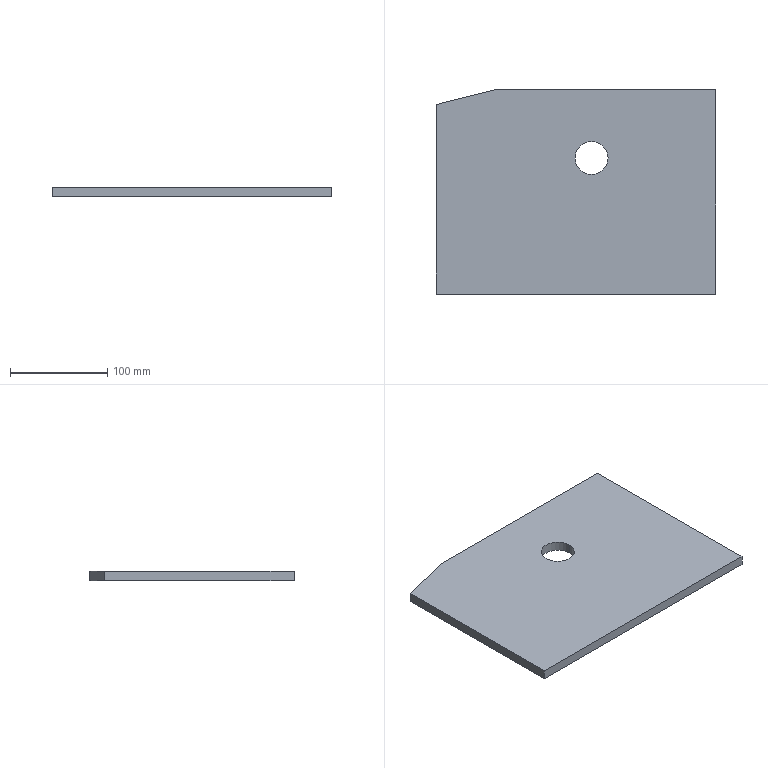Part | STEP file | 001-003-Shaft storage magazine side plate | 1 solid | 9 faces | box 288 x 210 x 10 mm | volume 591209 mm3 | plane 7 | cylinder 2 | commonest cylinder face diameters 34 x2
STEP:
#1=CARTESIAN_POINT('',(0.,0.,0.));
#2=DIRECTION('',(0.,0.,1.));
#3=DIRECTION('',(1.,0.,0.));
#4=AXIS2_PLACEMENT_3D('',#1,#2,#3);
#5=CARTESIAN_POINT('',(-1.,35.,10.));
#6=VERTEX_POINT('',#5);
#7=CARTESIAN_POINT('',(-1.,35.,0.));
#8=VERTEX_POINT('',#7);
#9=CARTESIAN_POINT('',(-1.,35.,10.));
#10=DIRECTION('',(0.,0.,-1.));
#11=VECTOR('',#10,1.);
#12=LINE('',#9,#11);
#13=CARTESIAN_POINT('',(16.,35.,10.));
#14=DIRECTION('',(0.,0.,-1.));
#15=DIRECTION('',(-1.,0.,0.));
#16=AXIS2_PLACEMENT_3D('',#13,#14,#15);
#17=CYLINDRICAL_SURFACE('',#16,17.);
#18=CARTESIAN_POINT('',(6.283,0.));
#19=DIRECTION('',(0.,1.));
#20=VECTOR('',#19,1.);
#21=LINE('',#18,#20);
#22=(GEOMETRIC_REPRESENTATION_CONTEXT(2)PARAMETRIC_REPRESENTATION_CONTEXT()REPRESENTATION_CONTEXT('',''));
#23=DEFINITIONAL_REPRESENTATION('',(#21),#22);
#24=PCURVE('',#17,#23);
#25=CARTESIAN_POINT('',(16.,35.,10.));
#26=DIRECTION('',(0.,0.,-1.));
#27=DIRECTION('',(-1.,0.,0.));
#28=AXIS2_PLACEMENT_3D('',#25,#26,#27);
#29=CYLINDRICAL_SURFACE('',#28,17.);
#30=CARTESIAN_POINT('',(0.,0.));
#31=DIRECTION('',(0.,1.));
#32=VECTOR('',#31,1.);
#33=LINE('',#30,#32);
#34=(GEOMETRIC_REPRESENTATION_CONTEXT(2)PARAMETRIC_REPRESENTATION_CONTEXT()REPRESENTATION_CONTEXT('',''));
#35=DEFINITIONAL_REPRESENTATION('',(#33),#34);
#36=PCURVE('',#29,#35);
#37=SURFACE_CURVE('',#12,(#24,#36),.PCURVE_S1.);
#38=EDGE_CURVE('',#6,#8,#37,.T.);
#39=ORIENTED_EDGE('',*,*,#38,.T.);
#40=CARTESIAN_POINT('',(33.,35.,0.));
#41=VERTEX_POINT('',#40);
#42=CARTESIAN_POINT('',(16.,35.,0.));
#43=DIRECTION('',(0.,0.,-1.));
#44=DIRECTION('',(-1.,0.,0.));
#45=AXIS2_PLACEMENT_3D('',#42,#43,#44);
#46=CIRCLE('',#45,17.);
#47=CARTESIAN_POINT('',(0.,10.));
#48=DIRECTION('',(1.,0.));
#49=VECTOR('',#48,1.);
#50=LINE('',#47,#49);
#51=(GEOMETRIC_REPRESENTATION_CONTEXT(2)PARAMETRIC_REPRESENTATION_CONTEXT()REPRESENTATION_CONTEXT('',''));
#52=DEFINITIONAL_REPRESENTATION('',(#50),#51);
#53=PCURVE('',#17,#52);
#54=CARTESIAN_POINT('',(0.,0.,0.));
#55=DIRECTION('',(0.,0.,-1.));
#56=DIRECTION('',(-1.,0.,0.));
#57=AXIS2_PLACEMENT_3D('',#54,#55,#56);
#58=PLANE('',#57);
#59=CARTESIAN_POINT('',(-16.,35.));
#60=DIRECTION('',(1.,0.));
#61=AXIS2_PLACEMENT_2D('',#59,#60);
#62=CIRCLE('',#61,17.);
#63=(GEOMETRIC_REPRESENTATION_CONTEXT(2)PARAMETRIC_REPRESENTATION_CONTEXT()REPRESENTATION_CONTEXT('',''));
#64=DEFINITIONAL_REPRESENTATION('',(#62),#63);
#65=PCURVE('',#58,#64);
#66=SURFACE_CURVE('',#46,(#53,#65),.PCURVE_S1.);
#67=EDGE_CURVE('',#41,#8,#66,.T.);
#68=ORIENTED_EDGE('',*,*,#67,.F.);
#69=CARTESIAN_POINT('',(33.,35.,10.));
#70=VERTEX_POINT('',#69);
#71=CARTESIAN_POINT('',(33.,35.,10.));
#72=DIRECTION('',(0.,0.,-1.));
#73=VECTOR('',#72,1.);
#74=LINE('',#71,#73);
#75=CARTESIAN_POINT('',(3.142,0.));
#76=DIRECTION('',(0.,1.));
#77=VECTOR('',#76,1.);
#78=LINE('',#75,#77);
#79=(GEOMETRIC_REPRESENTATION_CONTEXT(2)PARAMETRIC_REPRESENTATION_CONTEXT()REPRESENTATION_CONTEXT('',''));
#80=DEFINITIONAL_REPRESENTATION('',(#78),#79);
#81=PCURVE('',#17,#80);
#82=CARTESIAN_POINT('',(3.142,0.));
#83=DIRECTION('',(0.,1.));
#84=VECTOR('',#83,1.);
#85=LINE('',#82,#84);
#86=(GEOMETRIC_REPRESENTATION_CONTEXT(2)PARAMETRIC_REPRESENTATION_CONTEXT()REPRESENTATION_CONTEXT('',''));
#87=DEFINITIONAL_REPRESENTATION('',(#85),#86);
#88=PCURVE('',#29,#87);
#89=SURFACE_CURVE('',#74,(#81,#88),.PCURVE_S1.);
#90=EDGE_CURVE('',#70,#41,#89,.T.);
#91=ORIENTED_EDGE('',*,*,#90,.F.);
#92=CARTESIAN_POINT('',(16.,35.,10.));
#93=DIRECTION('',(0.,0.,-1.));
#94=DIRECTION('',(-1.,0.,0.));
#95=AXIS2_PLACEMENT_3D('',#92,#93,#94);
#96=CIRCLE('',#95,17.);
#97=CARTESIAN_POINT('',(0.,0.));
#98=DIRECTION('',(1.,0.));
#99=VECTOR('',#98,1.);
#100=LINE('',#97,#99);
#101=(GEOMETRIC_REPRESENTATION_CONTEXT(2)PARAMETRIC_REPRESENTATION_CONTEXT()REPRESENTATION_CONTEXT('',''));
#102=DEFINITIONAL_REPRESENTATION('',(#100),#101);
#103=PCURVE('',#17,#102);
#104=CARTESIAN_POINT('',(0.,0.,10.));
#105=DIRECTION('',(0.,0.,-1.));
#106=DIRECTION('',(-1.,0.,0.));
#107=AXIS2_PLACEMENT_3D('',#104,#105,#106);
#108=PLANE('',#107);
#109=CARTESIAN_POINT('',(-16.,35.));
#110=DIRECTION('',(1.,0.));
#111=AXIS2_PLACEMENT_2D('',#109,#110);
#112=CIRCLE('',#111,17.);
#113=(GEOMETRIC_REPRESENTATION_CONTEXT(2)PARAMETRIC_REPRESENTATION_CONTEXT()REPRESENTATION_CONTEXT('',''));
#114=DEFINITIONAL_REPRESENTATION('',(#112),#113);
#115=PCURVE('',#108,#114);
#116=SURFACE_CURVE('',#96,(#103,#115),.PCURVE_S1.);
#117=EDGE_CURVE('',#70,#6,#116,.T.);
#118=ORIENTED_EDGE('',*,*,#117,.T.);
#119=EDGE_LOOP('',(#39,#68,#91,#118));
#120=FACE_BOUND('',#119,.F.);
#121=ADVANCED_FACE('',(#120),#17,.F.);
#122=CARTESIAN_POINT('',(-83.838,105.,10.));
#123=VERTEX_POINT('',#122);
#124=CARTESIAN_POINT('',(-83.838,105.,0.));
#125=VERTEX_POINT('',#124);
#126=CARTESIAN_POINT('',(-83.838,105.,10.));
#127=DIRECTION('',(0.,0.,-1.));
#128=VECTOR('',#127,1.);
#129=LINE('',#126,#128);
#130=CARTESIAN_POINT('',(-144.,105.,10.));
#131=DIRECTION('',(0.,-1.,0.));
#132=DIRECTION('',(0.,0.,-1.));
#133=AXIS2_PLACEMENT_3D('',#130,#131,#132);
#134=PLANE('',#133);
#135=CARTESIAN_POINT('',(0.,60.162));
#136=DIRECTION('',(1.,0.));
#137=VECTOR('',#136,1.);
#138=LINE('',#135,#137);
#139=(GEOMETRIC_REPRESENTATION_CONTEXT(2)PARAMETRIC_REPRESENTATION_CONTEXT()REPRESENTATION_CONTEXT('',''));
#140=DEFINITIONAL_REPRESENTATION('',(#138),#139);
#141=PCURVE('',#134,#140);
#142=CARTESIAN_POINT('',(-83.838,105.,10.));
#143=DIRECTION('',(-0.2419,0.9703,0.));
#144=DIRECTION('',(-0.9703,-0.2419,0.));
#145=AXIS2_PLACEMENT_3D('',#142,#143,#144);
#146=PLANE('',#145);
#147=CARTESIAN_POINT('',(0.,0.));
#148=DIRECTION('',(0.,-1.));
#149=VECTOR('',#148,1.);
#150=LINE('',#147,#149);
#151=(GEOMETRIC_REPRESENTATION_CONTEXT(2)PARAMETRIC_REPRESENTATION_CONTEXT()REPRESENTATION_CONTEXT('',''));
#152=DEFINITIONAL_REPRESENTATION('',(#150),#151);
#153=PCURVE('',#146,#152);
#154=SURFACE_CURVE('',#129,(#141,#153),.PCURVE_S1.);
#155=EDGE_CURVE('',#123,#125,#154,.T.);
#156=ORIENTED_EDGE('',*,*,#155,.F.);
#157=CARTESIAN_POINT('',(144.,105.,10.));
#158=VERTEX_POINT('',#157);
#159=CARTESIAN_POINT('',(-144.,105.,10.));
#160=DIRECTION('',(-1.,0.,0.));
#161=VECTOR('',#160,1.);
#162=LINE('',#159,#161);
#163=CARTESIAN_POINT('',(0.,0.));
#164=DIRECTION('',(0.,-1.));
#165=VECTOR('',#164,1.);
#166=LINE('',#163,#165);
#167=(GEOMETRIC_REPRESENTATION_CONTEXT(2)PARAMETRIC_REPRESENTATION_CONTEXT()REPRESENTATION_CONTEXT('',''));
#168=DEFINITIONAL_REPRESENTATION('',(#166),#167);
#169=PCURVE('',#134,#168);
#170=CARTESIAN_POINT('',(144.,105.));
#171=DIRECTION('',(1.,0.));
#172=VECTOR('',#171,1.);
#173=LINE('',#170,#172);
#174=(GEOMETRIC_REPRESENTATION_CONTEXT(2)PARAMETRIC_REPRESENTATION_CONTEXT()REPRESENTATION_CONTEXT('',''));
#175=DEFINITIONAL_REPRESENTATION('',(#173),#174);
#176=PCURVE('',#108,#175);
#177=SURFACE_CURVE('',#162,(#169,#176),.PCURVE_S1.);
#178=EDGE_CURVE('',#158,#123,#177,.T.);
#179=ORIENTED_EDGE('',*,*,#178,.F.);
#180=CARTESIAN_POINT('',(144.,105.,0.));
#181=VERTEX_POINT('',#180);
#182=CARTESIAN_POINT('',(144.,105.,10.));
#183=DIRECTION('',(0.,0.,-1.));
#184=VECTOR('',#183,1.);
#185=LINE('',#182,#184);
#186=CARTESIAN_POINT('',(0.,288.));
#187=DIRECTION('',(1.,0.));
#188=VECTOR('',#187,1.);
#189=LINE('',#186,#188);
#190=(GEOMETRIC_REPRESENTATION_CONTEXT(2)PARAMETRIC_REPRESENTATION_CONTEXT()REPRESENTATION_CONTEXT('',''));
#191=DEFINITIONAL_REPRESENTATION('',(#189),#190);
#192=PCURVE('',#134,#191);
#193=CARTESIAN_POINT('',(144.,-105.,10.));
#194=DIRECTION('',(-1.,0.,0.));
#195=DIRECTION('',(0.,0.,1.));
#196=AXIS2_PLACEMENT_3D('',#193,#194,#195);
#197=PLANE('',#196);
#198=CARTESIAN_POINT('',(0.,210.));
#199=DIRECTION('',(-1.,0.));
#200=VECTOR('',#199,1.);
#201=LINE('',#198,#200);
#202=(GEOMETRIC_REPRESENTATION_CONTEXT(2)PARAMETRIC_REPRESENTATION_CONTEXT()REPRESENTATION_CONTEXT('',''));
#203=DEFINITIONAL_REPRESENTATION('',(#201),#202);
#204=PCURVE('',#197,#203);
#205=SURFACE_CURVE('',#185,(#192,#204),.PCURVE_S1.);
#206=EDGE_CURVE('',#158,#181,#205,.T.);
#207=ORIENTED_EDGE('',*,*,#206,.T.);
#208=CARTESIAN_POINT('',(-144.,105.,0.));
#209=DIRECTION('',(-1.,0.,0.));
#210=VECTOR('',#209,1.);
#211=LINE('',#208,#210);
#212=CARTESIAN_POINT('',(10.,0.));
#213=DIRECTION('',(0.,-1.));
#214=VECTOR('',#213,1.);
#215=LINE('',#212,#214);
#216=(GEOMETRIC_REPRESENTATION_CONTEXT(2)PARAMETRIC_REPRESENTATION_CONTEXT()REPRESENTATION_CONTEXT('',''));
#217=DEFINITIONAL_REPRESENTATION('',(#215),#216);
#218=PCURVE('',#134,#217);
#219=CARTESIAN_POINT('',(144.,105.));
#220=DIRECTION('',(1.,0.));
#221=VECTOR('',#220,1.);
#222=LINE('',#219,#221);
#223=(GEOMETRIC_REPRESENTATION_CONTEXT(2)PARAMETRIC_REPRESENTATION_CONTEXT()REPRESENTATION_CONTEXT('',''));
#224=DEFINITIONAL_REPRESENTATION('',(#222),#223);
#225=PCURVE('',#58,#224);
#226=SURFACE_CURVE('',#211,(#218,#225),.PCURVE_S1.);
#227=EDGE_CURVE('',#181,#125,#226,.T.);
#228=ORIENTED_EDGE('',*,*,#227,.T.);
#229=EDGE_LOOP('',(#156,#179,#207,#228));
#230=FACE_BOUND('',#229,.T.);
#231=ADVANCED_FACE('',(#230),#134,.F.);
#232=CARTESIAN_POINT('',(-144.,90.,10.));
#233=VERTEX_POINT('',#232);
#234=CARTESIAN_POINT('',(-144.,90.,0.));
#235=VERTEX_POINT('',#234);
#236=CARTESIAN_POINT('',(-144.,90.,10.));
#237=DIRECTION('',(0.,0.,-1.));
#238=VECTOR('',#237,1.);
#239=LINE('',#236,#238);
#240=CARTESIAN_POINT('',(-144.,-105.,10.));
#241=DIRECTION('',(1.,0.,0.));
#242=DIRECTION('',(0.,0.,-1.));
#243=AXIS2_PLACEMENT_3D('',#240,#241,#242);
#244=PLANE('',#243);
#245=CARTESIAN_POINT('',(0.,195.));
#246=DIRECTION('',(1.,0.));
#247=VECTOR('',#246,1.);
#248=LINE('',#245,#247);
#249=(GEOMETRIC_REPRESENTATION_CONTEXT(2)PARAMETRIC_REPRESENTATION_CONTEXT()REPRESENTATION_CONTEXT('',''));
#250=DEFINITIONAL_REPRESENTATION('',(#248),#249);
#251=PCURVE('',#244,#250);
#252=CARTESIAN_POINT('',(62.003,0.));
#253=DIRECTION('',(0.,-1.));
#254=VECTOR('',#253,1.);
#255=LINE('',#252,#254);
#256=(GEOMETRIC_REPRESENTATION_CONTEXT(2)PARAMETRIC_REPRESENTATION_CONTEXT()REPRESENTATION_CONTEXT('',''));
#257=DEFINITIONAL_REPRESENTATION('',(#255),#256);
#258=PCURVE('',#146,#257);
#259=SURFACE_CURVE('',#239,(#251,#258),.PCURVE_S1.);
#260=EDGE_CURVE('',#233,#235,#259,.T.);
#261=ORIENTED_EDGE('',*,*,#260,.T.);
#262=CARTESIAN_POINT('',(-144.,-105.,0.));
#263=VERTEX_POINT('',#262);
#264=CARTESIAN_POINT('',(-144.,-105.,0.));
#265=DIRECTION('',(0.,-1.,0.));
#266=VECTOR('',#265,1.);
#267=LINE('',#264,#266);
#268=CARTESIAN_POINT('',(10.,0.));
#269=DIRECTION('',(0.,-1.));
#270=VECTOR('',#269,1.);
#271=LINE('',#268,#270);
#272=(GEOMETRIC_REPRESENTATION_CONTEXT(2)PARAMETRIC_REPRESENTATION_CONTEXT()REPRESENTATION_CONTEXT('',''));
#273=DEFINITIONAL_REPRESENTATION('',(#271),#272);
#274=PCURVE('',#244,#273);
#275=CARTESIAN_POINT('',(144.,-105.));
#276=DIRECTION('',(0.,-1.));
#277=VECTOR('',#276,1.);
#278=LINE('',#275,#277);
#279=(GEOMETRIC_REPRESENTATION_CONTEXT(2)PARAMETRIC_REPRESENTATION_CONTEXT()REPRESENTATION_CONTEXT('',''));
#280=DEFINITIONAL_REPRESENTATION('',(#278),#279);
#281=PCURVE('',#58,#280);
#282=SURFACE_CURVE('',#267,(#274,#281),.PCURVE_S1.);
#283=EDGE_CURVE('',#235,#263,#282,.T.);
#284=ORIENTED_EDGE('',*,*,#283,.T.);
#285=CARTESIAN_POINT('',(-144.,-105.,10.));
#286=VERTEX_POINT('',#285);
#287=CARTESIAN_POINT('',(-144.,-105.,10.));
#288=DIRECTION('',(0.,0.,-1.));
#289=VECTOR('',#288,1.);
#290=LINE('',#287,#289);
#291=CARTESIAN_POINT('',(0.,0.));
#292=DIRECTION('',(1.,0.));
#293=VECTOR('',#292,1.);
#294=LINE('',#291,#293);
#295=(GEOMETRIC_REPRESENTATION_CONTEXT(2)PARAMETRIC_REPRESENTATION_CONTEXT()REPRESENTATION_CONTEXT('',''));
#296=DEFINITIONAL_REPRESENTATION('',(#294),#295);
#297=PCURVE('',#244,#296);
#298=CARTESIAN_POINT('',(-144.,-105.,10.));
#299=DIRECTION('',(0.,1.,0.));
#300=DIRECTION('',(0.,0.,1.));
#301=AXIS2_PLACEMENT_3D('',#298,#299,#300);
#302=PLANE('',#301);
#303=CARTESIAN_POINT('',(0.,0.));
#304=DIRECTION('',(-1.,0.));
#305=VECTOR('',#304,1.);
#306=LINE('',#303,#305);
#307=(GEOMETRIC_REPRESENTATION_CONTEXT(2)PARAMETRIC_REPRESENTATION_CONTEXT()REPRESENTATION_CONTEXT('',''));
#308=DEFINITIONAL_REPRESENTATION('',(#306),#307);
#309=PCURVE('',#302,#308);
#310=SURFACE_CURVE('',#290,(#297,#309),.PCURVE_S1.);
#311=EDGE_CURVE('',#286,#263,#310,.T.);
#312=ORIENTED_EDGE('',*,*,#311,.F.);
#313=CARTESIAN_POINT('',(-144.,-105.,10.));
#314=DIRECTION('',(0.,-1.,0.));
#315=VECTOR('',#314,1.);
#316=LINE('',#313,#315);
#317=CARTESIAN_POINT('',(0.,0.));
#318=DIRECTION('',(0.,-1.));
#319=VECTOR('',#318,1.);
#320=LINE('',#317,#319);
#321=(GEOMETRIC_REPRESENTATION_CONTEXT(2)PARAMETRIC_REPRESENTATION_CONTEXT()REPRESENTATION_CONTEXT('',''));
#322=DEFINITIONAL_REPRESENTATION('',(#320),#321);
#323=PCURVE('',#244,#322);
#324=CARTESIAN_POINT('',(144.,-105.));
#325=DIRECTION('',(0.,-1.));
#326=VECTOR('',#325,1.);
#327=LINE('',#324,#326);
#328=(GEOMETRIC_REPRESENTATION_CONTEXT(2)PARAMETRIC_REPRESENTATION_CONTEXT()REPRESENTATION_CONTEXT('',''));
#329=DEFINITIONAL_REPRESENTATION('',(#327),#328);
#330=PCURVE('',#108,#329);
#331=SURFACE_CURVE('',#316,(#323,#330),.PCURVE_S1.);
#332=EDGE_CURVE('',#233,#286,#331,.T.);
#333=ORIENTED_EDGE('',*,*,#332,.F.);
#334=EDGE_LOOP('',(#261,#284,#312,#333));
#335=FACE_BOUND('',#334,.T.);
#336=ADVANCED_FACE('',(#335),#244,.F.);
#337=CARTESIAN_POINT('',(16.,35.,10.));
#338=DIRECTION('',(0.,0.,-1.));
#339=DIRECTION('',(-1.,0.,0.));
#340=AXIS2_PLACEMENT_3D('',#337,#338,#339);
#341=CIRCLE('',#340,17.);
#342=CARTESIAN_POINT('',(-16.,35.));
#343=DIRECTION('',(1.,0.));
#344=AXIS2_PLACEMENT_2D('',#342,#343);
#345=CIRCLE('',#344,17.);
#346=(GEOMETRIC_REPRESENTATION_CONTEXT(2)PARAMETRIC_REPRESENTATION_CONTEXT()REPRESENTATION_CONTEXT('',''));
#347=DEFINITIONAL_REPRESENTATION('',(#345),#346);
#348=PCURVE('',#108,#347);
#349=CARTESIAN_POINT('',(0.,0.));
#350=DIRECTION('',(1.,0.));
#351=VECTOR('',#350,1.);
#352=LINE('',#349,#351);
#353=(GEOMETRIC_REPRESENTATION_CONTEXT(2)PARAMETRIC_REPRESENTATION_CONTEXT()REPRESENTATION_CONTEXT('',''));
#354=DEFINITIONAL_REPRESENTATION('',(#352),#353);
#355=PCURVE('',#29,#354);
#356=SURFACE_CURVE('',#341,(#348,#355),.PCURVE_S1.);
#357=EDGE_CURVE('',#6,#70,#356,.T.);
#358=ORIENTED_EDGE('',*,*,#357,.T.);
#359=ORIENTED_EDGE('',*,*,#117,.T.);
#360=EDGE_LOOP('',(#358,#359));
#361=FACE_BOUND('',#360,.T.);
#362=CARTESIAN_POINT('',(-83.838,105.,10.));
#363=DIRECTION('',(0.9703,0.2419,0.));
#364=VECTOR('',#363,1.);
#365=LINE('',#362,#364);
#366=CARTESIAN_POINT('',(83.838,105.));
#367=DIRECTION('',(-0.9703,0.2419));
#368=VECTOR('',#367,1.);
#369=LINE('',#366,#368);
#370=(GEOMETRIC_REPRESENTATION_CONTEXT(2)PARAMETRIC_REPRESENTATION_CONTEXT()REPRESENTATION_CONTEXT('',''));
#371=DEFINITIONAL_REPRESENTATION('',(#369),#370);
#372=PCURVE('',#108,#371);
#373=CARTESIAN_POINT('',(0.,0.));
#374=DIRECTION('',(-1.,0.));
#375=VECTOR('',#374,1.);
#376=LINE('',#373,#375);
#377=(GEOMETRIC_REPRESENTATION_CONTEXT(2)PARAMETRIC_REPRESENTATION_CONTEXT()REPRESENTATION_CONTEXT('',''));
#378=DEFINITIONAL_REPRESENTATION('',(#376),#377);
#379=PCURVE('',#146,#378);
#380=SURFACE_CURVE('',#365,(#372,#379),.PCURVE_S1.);
#381=EDGE_CURVE('',#233,#123,#380,.T.);
#382=ORIENTED_EDGE('',*,*,#381,.F.);
#383=ORIENTED_EDGE('',*,*,#332,.T.);
#384=CARTESIAN_POINT('',(144.,-105.,10.));
#385=VERTEX_POINT('',#384);
#386=CARTESIAN_POINT('',(-144.,-105.,10.));
#387=DIRECTION('',(1.,0.,0.));
#388=VECTOR('',#387,1.);
#389=LINE('',#386,#388);
#390=CARTESIAN_POINT('',(144.,-105.));
#391=DIRECTION('',(-1.,0.));
#392=VECTOR('',#391,1.);
#393=LINE('',#390,#392);
#394=(GEOMETRIC_REPRESENTATION_CONTEXT(2)PARAMETRIC_REPRESENTATION_CONTEXT()REPRESENTATION_CONTEXT('',''));
#395=DEFINITIONAL_REPRESENTATION('',(#393),#394);
#396=PCURVE('',#108,#395);
#397=CARTESIAN_POINT('',(0.,0.));
#398=DIRECTION('',(0.,1.));
#399=VECTOR('',#398,1.);
#400=LINE('',#397,#399);
#401=(GEOMETRIC_REPRESENTATION_CONTEXT(2)PARAMETRIC_REPRESENTATION_CONTEXT()REPRESENTATION_CONTEXT('',''));
#402=DEFINITIONAL_REPRESENTATION('',(#400),#401);
#403=PCURVE('',#302,#402);
#404=SURFACE_CURVE('',#389,(#396,#403),.PCURVE_S1.);
#405=EDGE_CURVE('',#286,#385,#404,.T.);
#406=ORIENTED_EDGE('',*,*,#405,.T.);
#407=CARTESIAN_POINT('',(144.,-105.,10.));
#408=DIRECTION('',(0.,1.,0.));
#409=VECTOR('',#408,1.);
#410=LINE('',#407,#409);
#411=CARTESIAN_POINT('',(-144.,-105.));
#412=DIRECTION('',(0.,1.));
#413=VECTOR('',#412,1.);
#414=LINE('',#411,#413);
#415=(GEOMETRIC_REPRESENTATION_CONTEXT(2)PARAMETRIC_REPRESENTATION_CONTEXT()REPRESENTATION_CONTEXT('',''));
#416=DEFINITIONAL_REPRESENTATION('',(#414),#415);
#417=PCURVE('',#108,#416);
#418=CARTESIAN_POINT('',(0.,0.));
#419=DIRECTION('',(0.,1.));
#420=VECTOR('',#419,1.);
#421=LINE('',#418,#420);
#422=(GEOMETRIC_REPRESENTATION_CONTEXT(2)PARAMETRIC_REPRESENTATION_CONTEXT()REPRESENTATION_CONTEXT('',''));
#423=DEFINITIONAL_REPRESENTATION('',(#421),#422);
#424=PCURVE('',#197,#423);
#425=SURFACE_CURVE('',#410,(#417,#424),.PCURVE_S1.);
#426=EDGE_CURVE('',#385,#158,#425,.T.);
#427=ORIENTED_EDGE('',*,*,#426,.T.);
#428=ORIENTED_EDGE('',*,*,#178,.T.);
#429=EDGE_LOOP('',(#382,#383,#406,#427,#428));
#430=FACE_BOUND('',#429,.T.);
#431=ADVANCED_FACE('',(#361,#430),#108,.F.);
#432=CARTESIAN_POINT('',(16.,35.,0.));
#433=DIRECTION('',(0.,0.,-1.));
#434=DIRECTION('',(-1.,0.,0.));
#435=AXIS2_PLACEMENT_3D('',#432,#433,#434);
#436=CIRCLE('',#435,17.);
#437=CARTESIAN_POINT('',(-16.,35.));
#438=DIRECTION('',(1.,0.));
#439=AXIS2_PLACEMENT_2D('',#437,#438);
#440=CIRCLE('',#439,17.);
#441=(GEOMETRIC_REPRESENTATION_CONTEXT(2)PARAMETRIC_REPRESENTATION_CONTEXT()REPRESENTATION_CONTEXT('',''));
#442=DEFINITIONAL_REPRESENTATION('',(#440),#441);
#443=PCURVE('',#58,#442);
#444=CARTESIAN_POINT('',(0.,10.));
#445=DIRECTION('',(1.,0.));
#446=VECTOR('',#445,1.);
#447=LINE('',#444,#446);
#448=(GEOMETRIC_REPRESENTATION_CONTEXT(2)PARAMETRIC_REPRESENTATION_CONTEXT()REPRESENTATION_CONTEXT('',''));
#449=DEFINITIONAL_REPRESENTATION('',(#447),#448);
#450=PCURVE('',#29,#449);
#451=SURFACE_CURVE('',#436,(#443,#450),.PCURVE_S1.);
#452=EDGE_CURVE('',#8,#41,#451,.T.);
#453=ORIENTED_EDGE('',*,*,#452,.F.);
#454=ORIENTED_EDGE('',*,*,#67,.F.);
#455=EDGE_LOOP('',(#453,#454));
#456=FACE_BOUND('',#455,.T.);
#457=ORIENTED_EDGE('',*,*,#283,.F.);
#458=CARTESIAN_POINT('',(-83.838,105.,0.));
#459=DIRECTION('',(0.9703,0.2419,0.));
#460=VECTOR('',#459,1.);
#461=LINE('',#458,#460);
#462=CARTESIAN_POINT('',(83.838,105.));
#463=DIRECTION('',(-0.9703,0.2419));
#464=VECTOR('',#463,1.);
#465=LINE('',#462,#464);
#466=(GEOMETRIC_REPRESENTATION_CONTEXT(2)PARAMETRIC_REPRESENTATION_CONTEXT()REPRESENTATION_CONTEXT('',''));
#467=DEFINITIONAL_REPRESENTATION('',(#465),#466);
#468=PCURVE('',#58,#467);
#469=CARTESIAN_POINT('',(0.,-10.));
#470=DIRECTION('',(-1.,0.));
#471=VECTOR('',#470,1.);
#472=LINE('',#469,#471);
#473=(GEOMETRIC_REPRESENTATION_CONTEXT(2)PARAMETRIC_REPRESENTATION_CONTEXT()REPRESENTATION_CONTEXT('',''));
#474=DEFINITIONAL_REPRESENTATION('',(#472),#473);
#475=PCURVE('',#146,#474);
#476=SURFACE_CURVE('',#461,(#468,#475),.PCURVE_S1.);
#477=EDGE_CURVE('',#235,#125,#476,.T.);
#478=ORIENTED_EDGE('',*,*,#477,.T.);
#479=ORIENTED_EDGE('',*,*,#227,.F.);
#480=CARTESIAN_POINT('',(144.,-105.,0.));
#481=VERTEX_POINT('',#480);
#482=CARTESIAN_POINT('',(144.,-105.,0.));
#483=DIRECTION('',(0.,1.,0.));
#484=VECTOR('',#483,1.);
#485=LINE('',#482,#484);
#486=CARTESIAN_POINT('',(-144.,-105.));
#487=DIRECTION('',(0.,1.));
#488=VECTOR('',#487,1.);
#489=LINE('',#486,#488);
#490=(GEOMETRIC_REPRESENTATION_CONTEXT(2)PARAMETRIC_REPRESENTATION_CONTEXT()REPRESENTATION_CONTEXT('',''));
#491=DEFINITIONAL_REPRESENTATION('',(#489),#490);
#492=PCURVE('',#58,#491);
#493=CARTESIAN_POINT('',(-10.,0.));
#494=DIRECTION('',(0.,1.));
#495=VECTOR('',#494,1.);
#496=LINE('',#493,#495);
#497=(GEOMETRIC_REPRESENTATION_CONTEXT(2)PARAMETRIC_REPRESENTATION_CONTEXT()REPRESENTATION_CONTEXT('',''));
#498=DEFINITIONAL_REPRESENTATION('',(#496),#497);
#499=PCURVE('',#197,#498);
#500=SURFACE_CURVE('',#485,(#492,#499),.PCURVE_S1.);
#501=EDGE_CURVE('',#481,#181,#500,.T.);
#502=ORIENTED_EDGE('',*,*,#501,.F.);
#503=CARTESIAN_POINT('',(-144.,-105.,0.));
#504=DIRECTION('',(1.,0.,0.));
#505=VECTOR('',#504,1.);
#506=LINE('',#503,#505);
#507=CARTESIAN_POINT('',(144.,-105.));
#508=DIRECTION('',(-1.,0.));
#509=VECTOR('',#508,1.);
#510=LINE('',#507,#509);
#511=(GEOMETRIC_REPRESENTATION_CONTEXT(2)PARAMETRIC_REPRESENTATION_CONTEXT()REPRESENTATION_CONTEXT('',''));
#512=DEFINITIONAL_REPRESENTATION('',(#510),#511);
#513=PCURVE('',#58,#512);
#514=CARTESIAN_POINT('',(-10.,0.));
#515=DIRECTION('',(0.,1.));
#516=VECTOR('',#515,1.);
#517=LINE('',#514,#516);
#518=(GEOMETRIC_REPRESENTATION_CONTEXT(2)PARAMETRIC_REPRESENTATION_CONTEXT()REPRESENTATION_CONTEXT('',''));
#519=DEFINITIONAL_REPRESENTATION('',(#517),#518);
#520=PCURVE('',#302,#519);
#521=SURFACE_CURVE('',#506,(#513,#520),.PCURVE_S1.);
#522=EDGE_CURVE('',#263,#481,#521,.T.);
#523=ORIENTED_EDGE('',*,*,#522,.F.);
#524=EDGE_LOOP('',(#457,#478,#479,#502,#523));
#525=FACE_BOUND('',#524,.T.);
#526=ADVANCED_FACE('',(#456,#525),#58,.T.);
#527=ORIENTED_EDGE('',*,*,#501,.T.);
#528=ORIENTED_EDGE('',*,*,#206,.F.);
#529=ORIENTED_EDGE('',*,*,#426,.F.);
#530=CARTESIAN_POINT('',(144.,-105.,10.));
#531=DIRECTION('',(0.,0.,-1.));
#532=VECTOR('',#531,1.);
#533=LINE('',#530,#532);
#534=CARTESIAN_POINT('',(0.,0.));
#535=DIRECTION('',(-1.,0.));
#536=VECTOR('',#535,1.);
#537=LINE('',#534,#536);
#538=(GEOMETRIC_REPRESENTATION_CONTEXT(2)PARAMETRIC_REPRESENTATION_CONTEXT()REPRESENTATION_CONTEXT('',''));
#539=DEFINITIONAL_REPRESENTATION('',(#537),#538);
#540=PCURVE('',#197,#539);
#541=CARTESIAN_POINT('',(0.,288.));
#542=DIRECTION('',(-1.,0.));
#543=VECTOR('',#542,1.);
#544=LINE('',#541,#543);
#545=(GEOMETRIC_REPRESENTATION_CONTEXT(2)PARAMETRIC_REPRESENTATION_CONTEXT()REPRESENTATION_CONTEXT('',''));
#546=DEFINITIONAL_REPRESENTATION('',(#544),#545);
#547=PCURVE('',#302,#546);
#548=SURFACE_CURVE('',#533,(#540,#547),.PCURVE_S1.);
#549=EDGE_CURVE('',#385,#481,#548,.T.);
#550=ORIENTED_EDGE('',*,*,#549,.T.);
#551=EDGE_LOOP('',(#527,#528,#529,#550));
#552=FACE_BOUND('',#551,.T.);
#553=ADVANCED_FACE('',(#552),#197,.F.);
#554=ORIENTED_EDGE('',*,*,#522,.T.);
#555=ORIENTED_EDGE('',*,*,#549,.F.);
#556=ORIENTED_EDGE('',*,*,#405,.F.);
#557=ORIENTED_EDGE('',*,*,#311,.T.);
#558=EDGE_LOOP('',(#554,#555,#556,#557));
#559=FACE_BOUND('',#558,.T.);
#560=ADVANCED_FACE('',(#559),#302,.F.);
#561=ORIENTED_EDGE('',*,*,#477,.F.);
#562=ORIENTED_EDGE('',*,*,#260,.F.);
#563=ORIENTED_EDGE('',*,*,#381,.T.);
#564=ORIENTED_EDGE('',*,*,#155,.T.);
#565=EDGE_LOOP('',(#561,#562,#563,#564));
#566=FACE_BOUND('',#565,.T.);
#567=ADVANCED_FACE('',(#566),#146,.T.);
#568=ORIENTED_EDGE('',*,*,#452,.F.);
#569=ORIENTED_EDGE('',*,*,#38,.F.);
#570=ORIENTED_EDGE('',*,*,#357,.T.);
#571=ORIENTED_EDGE('',*,*,#90,.T.);
#572=EDGE_LOOP('',(#568,#569,#570,#571));
#573=FACE_BOUND('',#572,.F.);
#574=ADVANCED_FACE('',(#573),#29,.F.);
#575=CLOSED_SHELL('',(#121,#231,#336,#431,#526,#553,#560,#567,#574));
#576=MANIFOLD_SOLID_BREP('',#575);
#577=(LENGTH_UNIT()NAMED_UNIT(*)SI_UNIT(.MILLI.,.METRE.));
#578=UNCERTAINTY_MEASURE_WITH_UNIT(LENGTH_MEASURE(0.0000001),#577,'','');
#579=(NAMED_UNIT(*)PLANE_ANGLE_UNIT()SI_UNIT($,.RADIAN.));
#580=(NAMED_UNIT(*)SI_UNIT($,.STERADIAN.)SOLID_ANGLE_UNIT());
#581=(GEOMETRIC_REPRESENTATION_CONTEXT(3)GLOBAL_UNCERTAINTY_ASSIGNED_CONTEXT((#578))GLOBAL_UNIT_ASSIGNED_CONTEXT((#577,#579,#580))REPRESENTATION_CONTEXT('',''));
#582=ADVANCED_BREP_SHAPE_REPRESENTATION('',(#4,#576),#581);